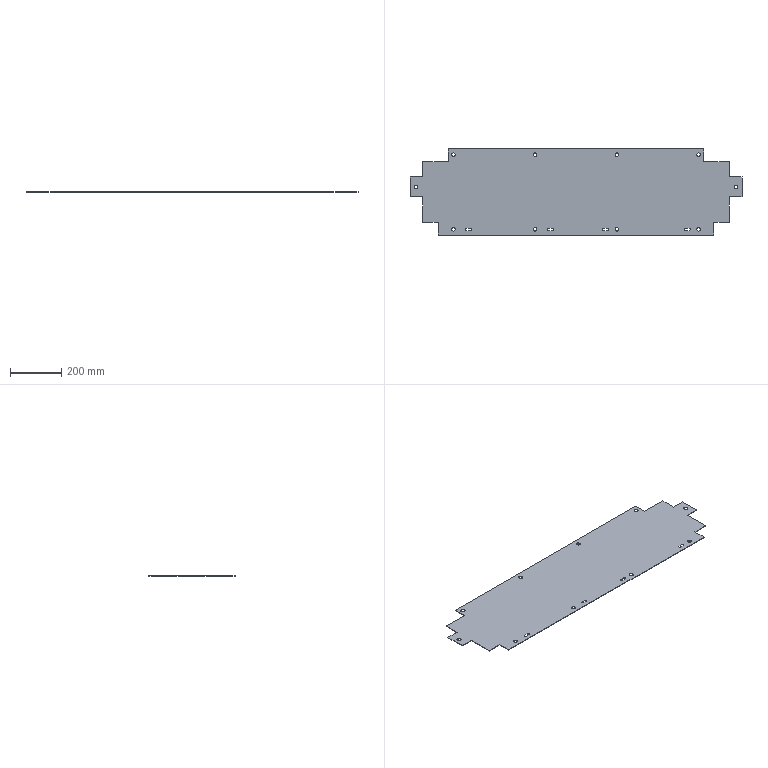Part | STEP file | Jig plate | 1 solid | 62 faces | box 1300 x 337.75 x 2 mm | volume 788863 mm3 | plane 30 | cone 20 | cylinder 12 | commonest cylinder face diameters 9 x12